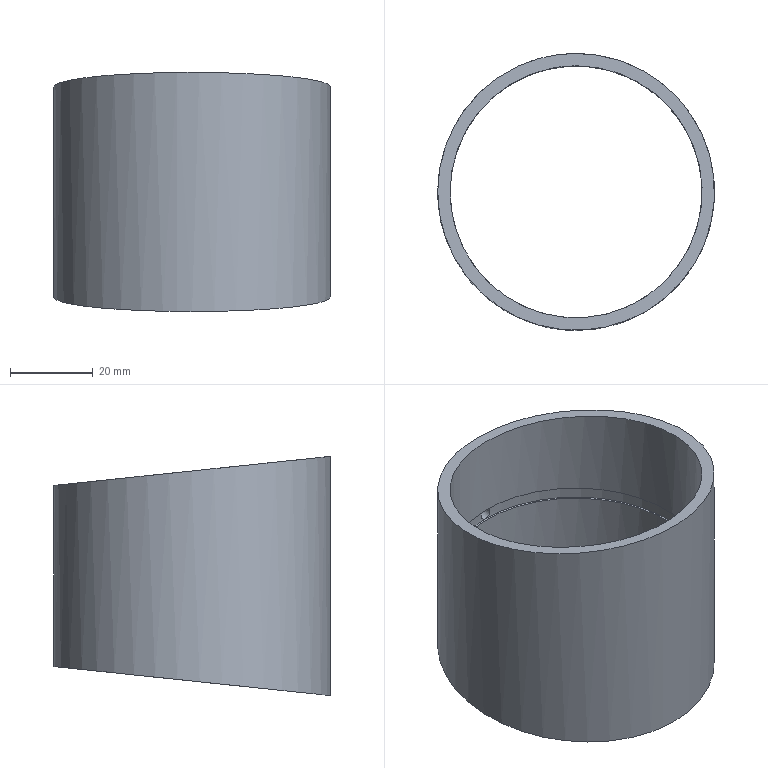Part | NX | features DATUM_CSYS 5, EXTRUDE 4, SKETCH 4, DATUM_PLANE 2, HOLE PACKAGE 1, MIRROR_SET 1, SIMPLE HOLE 1 | 1 solid | 9 faces | box 67 x 67 x 57.889 mm | volume 30363 mm3 | cylinder 5 | plane 4 | commonest cylinder face diameters 61 x2 3 x1 62 x1 67 x1
STEP:
#1=CARTESIAN_POINT('',(0.,30.5,52.218));
#2=VERTEX_POINT('',#1);
#3=CARTESIAN_POINT('',(0.,0.,55.423));
#4=DIRECTION('',(0.,-0.1045,-0.9945));
#5=DIRECTION('',(0.,0.9945,-0.1045));
#6=AXIS2_PLACEMENT_3D('',#3,#4,#5);
#7=ELLIPSE('',#6,30.668,30.5);
#8=EDGE_CURVE('',#2,#2,#7,.T.);
#9=ORIENTED_EDGE('',*,*,#8,.F.);
#10=EDGE_LOOP('',(#9));
#11=FACE_BOUND('',#10,.T.);
#12=CARTESIAN_POINT('',(-30.5,0.,32.));
#13=VERTEX_POINT('',#12);
#14=CARTESIAN_POINT('',(0.,0.,32.));
#15=DIRECTION('',(0.,0.,-1.));
#16=DIRECTION('',(-1.,0.,0.));
#17=AXIS2_PLACEMENT_3D('',#14,#15,#16);
#18=CIRCLE('',#17,30.5);
#19=EDGE_CURVE('',#13,#13,#18,.T.);
#20=ORIENTED_EDGE('',*,*,#19,.T.);
#21=EDGE_LOOP('',(#20));
#22=FACE_BOUND('',#21,.T.);
#23=CARTESIAN_POINT('',(0.,0.,60.));
#24=DIRECTION('',(0.,0.,-1.));
#25=DIRECTION('',(-1.,0.,0.));
#26=AXIS2_PLACEMENT_3D('',#23,#24,#25);
#27=CYLINDRICAL_SURFACE('',#26,30.5);
#28=ADVANCED_FACE('',(#11,#22),#27,.F.);
#29=CARTESIAN_POINT('',(1.5,33.466,30.5));
#30=VERTEX_POINT('',#29);
#31=CARTESIAN_POINT('',(1.174,33.483,29.323));
#32=CARTESIAN_POINT('',(1.663,33.458,30.5));
#33=CARTESIAN_POINT('',(1.175,33.483,31.676));
#34=CARTESIAN_POINT('',(0.001228,33.508,32.162));
#35=CARTESIAN_POINT('',(-1.175,33.483,31.676));
#36=CARTESIAN_POINT('',(-1.662,33.458,30.5));
#37=CARTESIAN_POINT('',(-1.177,33.483,29.326));
#38=CARTESIAN_POINT('',(-0.001751,33.508,28.838));
#39=CARTESIAN_POINT('',(1.174,33.483,29.323));
#40=CARTESIAN_POINT('',(1.663,33.458,30.5));
#41=CARTESIAN_POINT('',(1.175,33.483,31.676));
#42=B_SPLINE_CURVE_WITH_KNOTS('',3,(#31,#32,#33,#34,#35,#36,#37,#38,#39,#40,#41),.UNSPECIFIED.,.T.,.F.,(1,1,1,1,1,1,1,1,1,1,1,1,1,1,1),(-0.003517,-0.002345,-0.001172,0.,0.001172,0.002345,0.003517,0.00469,0.005862,0.007035,0.008207,0.009379,0.01055,0.01172,0.0129),.UNSPECIFIED.);
#43=EDGE_CURVE('',#30,#30,#42,.T.);
#44=ORIENTED_EDGE('',*,*,#43,.T.);
#45=EDGE_LOOP('',(#44));
#46=FACE_BOUND('',#45,.T.);
#47=CARTESIAN_POINT('',(0.,-33.5,1.056));
#48=VERTEX_POINT('',#47);
#49=CARTESIAN_POINT('',(0.,0.,4.577));
#50=DIRECTION('',(0.,-0.1045,0.9945));
#51=DIRECTION('',(0.,-0.9945,-0.1045));
#52=AXIS2_PLACEMENT_3D('',#49,#50,#51);
#53=ELLIPSE('',#52,33.685,33.5);
#54=EDGE_CURVE('',#48,#48,#53,.T.);
#55=ORIENTED_EDGE('',*,*,#54,.T.);
#56=EDGE_LOOP('',(#55));
#57=FACE_BOUND('',#56,.T.);
#58=CARTESIAN_POINT('',(0.,33.5,51.902));
#59=VERTEX_POINT('',#58);
#60=CARTESIAN_POINT('',(0.,0.,55.423));
#61=DIRECTION('',(0.,-0.1045,-0.9945));
#62=DIRECTION('',(0.,0.9945,-0.1045));
#63=AXIS2_PLACEMENT_3D('',#60,#61,#62);
#64=ELLIPSE('',#63,33.685,33.5);
#65=EDGE_CURVE('',#59,#59,#64,.T.);
#66=ORIENTED_EDGE('',*,*,#65,.T.);
#67=EDGE_LOOP('',(#66));
#68=FACE_BOUND('',#67,.T.);
#69=CARTESIAN_POINT('',(0.,0.,60.));
#70=DIRECTION('',(0.,0.,-1.));
#71=DIRECTION('',(-1.,0.,0.));
#72=AXIS2_PLACEMENT_3D('',#69,#70,#71);
#73=CYLINDRICAL_SURFACE('',#72,33.5);
#74=ADVANCED_FACE('',(#46,#57,#68),#73,.T.);
#75=CARTESIAN_POINT('',(-30.5,0.,29.));
#76=VERTEX_POINT('',#75);
#77=CARTESIAN_POINT('',(0.,0.,29.));
#78=DIRECTION('',(0.,0.,-1.));
#79=DIRECTION('',(-1.,0.,0.));
#80=AXIS2_PLACEMENT_3D('',#77,#78,#79);
#81=CIRCLE('',#80,30.5);
#82=EDGE_CURVE('',#76,#76,#81,.T.);
#83=ORIENTED_EDGE('',*,*,#82,.F.);
#84=EDGE_LOOP('',(#83));
#85=FACE_BOUND('',#84,.T.);
#86=CARTESIAN_POINT('',(0.,-30.5,1.371));
#87=VERTEX_POINT('',#86);
#88=CARTESIAN_POINT('',(0.,0.,4.577));
#89=DIRECTION('',(0.,-0.1045,0.9945));
#90=DIRECTION('',(0.,-0.9945,-0.1045));
#91=AXIS2_PLACEMENT_3D('',#88,#89,#90);
#92=ELLIPSE('',#91,30.668,30.5);
#93=EDGE_CURVE('',#87,#87,#92,.T.);
#94=ORIENTED_EDGE('',*,*,#93,.F.);
#95=EDGE_LOOP('',(#94));
#96=FACE_BOUND('',#95,.T.);
#97=CARTESIAN_POINT('',(0.,0.,60.));
#98=DIRECTION('',(0.,0.,-1.));
#99=DIRECTION('',(-1.,0.,0.));
#100=AXIS2_PLACEMENT_3D('',#97,#98,#99);
#101=CYLINDRICAL_SURFACE('',#100,30.5);
#102=ADVANCED_FACE('',(#85,#96),#101,.F.);
#103=ORIENTED_EDGE('',*,*,#8,.T.);
#104=EDGE_LOOP('',(#103));
#105=FACE_BOUND('',#104,.T.);
#106=ORIENTED_EDGE('',*,*,#65,.F.);
#107=EDGE_LOOP('',(#106));
#108=FACE_BOUND('',#107,.T.);
#109=CARTESIAN_POINT('',(-60.,-43.544,60.));
#110=DIRECTION('',(0.,-0.1045,-0.9945));
#111=DIRECTION('',(0.,0.9945,-0.1045));
#112=AXIS2_PLACEMENT_3D('',#109,#110,#111);
#113=PLANE('',#112);
#114=ADVANCED_FACE('',(#105,#108),#113,.F.);
#115=ORIENTED_EDGE('',*,*,#93,.T.);
#116=EDGE_LOOP('',(#115));
#117=FACE_BOUND('',#116,.T.);
#118=ORIENTED_EDGE('',*,*,#54,.F.);
#119=EDGE_LOOP('',(#118));
#120=FACE_BOUND('',#119,.T.);
#121=CARTESIAN_POINT('',(-60.,-43.544,0.));
#122=DIRECTION('',(0.,-0.1045,0.9945));
#123=DIRECTION('',(0.,0.9945,0.1045));
#124=AXIS2_PLACEMENT_3D('',#121,#122,#123);
#125=PLANE('',#124);
#126=ADVANCED_FACE('',(#117,#120),#125,.F.);
#127=CARTESIAN_POINT('',(0.,31.,29.));
#128=VERTEX_POINT('',#127);
#129=CARTESIAN_POINT('',(0.,31.,32.));
#130=VERTEX_POINT('',#129);
#131=CARTESIAN_POINT('',(0.,31.,29.));
#132=CARTESIAN_POINT('',(0.3958,31.,29.));
#133=CARTESIAN_POINT('',(1.174,30.982,29.324));
#134=CARTESIAN_POINT('',(1.663,30.955,30.502));
#135=CARTESIAN_POINT('',(1.174,30.982,31.676));
#136=CARTESIAN_POINT('',(0.3913,31.,32.));
#137=CARTESIAN_POINT('',(0.,31.,32.));
#138=B_SPLINE_CURVE_WITH_KNOTS('',3,(#131,#132,#133,#134,#135,#136,#137),.UNSPECIFIED.,.F.,.F.,(4,1,1,1,4),(0.007036,0.008209,0.009381,0.01055,0.01173),.UNSPECIFIED.);
#139=EDGE_CURVE('',#128,#130,#138,.T.);
#140=ORIENTED_EDGE('',*,*,#139,.T.);
#141=CARTESIAN_POINT('',(0.,31.,32.));
#142=CARTESIAN_POINT('',(-0.3914,31.,32.));
#143=CARTESIAN_POINT('',(-1.176,30.982,31.675));
#144=CARTESIAN_POINT('',(-1.663,30.955,30.499));
#145=CARTESIAN_POINT('',(-1.174,30.982,29.325));
#146=CARTESIAN_POINT('',(-0.3959,31.,29.));
#147=CARTESIAN_POINT('',(0.,31.,29.));
#148=B_SPLINE_CURVE_WITH_KNOTS('',3,(#141,#142,#143,#144,#145,#146,#147),.UNSPECIFIED.,.F.,.F.,(4,1,1,1,4),(0.002346,0.003518,0.004691,0.005864,0.007036),.UNSPECIFIED.);
#149=EDGE_CURVE('',#130,#128,#148,.T.);
#150=ORIENTED_EDGE('',*,*,#149,.T.);
#151=EDGE_LOOP('',(#140,#150));
#152=FACE_BOUND('',#151,.T.);
#153=ORIENTED_EDGE('',*,*,#43,.F.);
#154=EDGE_LOOP('',(#153));
#155=FACE_BOUND('',#154,.T.);
#156=CARTESIAN_POINT('',(0.,35.,30.5));
#157=DIRECTION('',(0.,-1.,0.));
#158=DIRECTION('',(1.,0.,0.));
#159=AXIS2_PLACEMENT_3D('',#156,#157,#158);
#160=CYLINDRICAL_SURFACE('',#159,1.5);
#161=ADVANCED_FACE('',(#152,#155),#160,.F.);
#162=CARTESIAN_POINT('',(0.,0.,32.));
#163=DIRECTION('',(0.,0.,-1.));
#164=DIRECTION('',(1.,0.,0.));
#165=AXIS2_PLACEMENT_3D('',#162,#163,#164);
#166=CIRCLE('',#165,31.);
#167=EDGE_CURVE('',#130,#130,#166,.F.);
#168=ORIENTED_EDGE('',*,*,#167,.T.);
#169=ORIENTED_EDGE('',*,*,#139,.F.);
#170=CARTESIAN_POINT('',(0.,0.,29.));
#171=DIRECTION('',(0.,0.,-1.));
#172=DIRECTION('',(1.,0.,0.));
#173=AXIS2_PLACEMENT_3D('',#170,#171,#172);
#174=CIRCLE('',#173,31.);
#175=EDGE_CURVE('',#128,#128,#174,.F.);
#176=ORIENTED_EDGE('',*,*,#175,.F.);
#177=ORIENTED_EDGE('',*,*,#149,.F.);
#178=EDGE_LOOP('',(#168,#169,#176,#177));
#179=FACE_BOUND('',#178,.T.);
#180=CARTESIAN_POINT('',(0.,0.,32.));
#181=DIRECTION('',(0.,0.,-1.));
#182=DIRECTION('',(-1.,0.,0.));
#183=AXIS2_PLACEMENT_3D('',#180,#181,#182);
#184=CYLINDRICAL_SURFACE('',#183,31.);
#185=ADVANCED_FACE('',(#179),#184,.F.);
#186=ORIENTED_EDGE('',*,*,#167,.F.);
#187=EDGE_LOOP('',(#186));
#188=FACE_BOUND('',#187,.T.);
#189=ORIENTED_EDGE('',*,*,#19,.F.);
#190=EDGE_LOOP('',(#189));
#191=FACE_BOUND('',#190,.T.);
#192=CARTESIAN_POINT('',(0.,0.,32.));
#193=DIRECTION('',(0.,0.,-1.));
#194=DIRECTION('',(-1.,0.,0.));
#195=AXIS2_PLACEMENT_3D('',#192,#193,#194);
#196=PLANE('',#195);
#197=ADVANCED_FACE('',(#188,#191),#196,.T.);
#198=ORIENTED_EDGE('',*,*,#175,.T.);
#199=EDGE_LOOP('',(#198));
#200=FACE_BOUND('',#199,.T.);
#201=ORIENTED_EDGE('',*,*,#82,.T.);
#202=EDGE_LOOP('',(#201));
#203=FACE_BOUND('',#202,.T.);
#204=CARTESIAN_POINT('',(0.,0.,29.));
#205=DIRECTION('',(0.,0.,-1.));
#206=DIRECTION('',(-1.,0.,0.));
#207=AXIS2_PLACEMENT_3D('',#204,#205,#206);
#208=PLANE('',#207);
#209=ADVANCED_FACE('',(#200,#203),#208,.F.);
#210=CLOSED_SHELL('',(#28,#74,#102,#114,#126,#161,#185,#197,#209));
#211=MANIFOLD_SOLID_BREP('',#210);
#212=(LENGTH_UNIT()NAMED_UNIT(*)SI_UNIT(.MILLI.,.METRE.));
#213=UNCERTAINTY_MEASURE_WITH_UNIT(LENGTH_MEASURE(0.0508),#212,'','');
#214=(NAMED_UNIT(*)PLANE_ANGLE_UNIT()SI_UNIT($,.RADIAN.));
#215=(NAMED_UNIT(*)SI_UNIT($,.STERADIAN.)SOLID_ANGLE_UNIT());
#216=(GEOMETRIC_REPRESENTATION_CONTEXT(3)GLOBAL_UNCERTAINTY_ASSIGNED_CONTEXT((#213))GLOBAL_UNIT_ASSIGNED_CONTEXT((#212,#214,#215))REPRESENTATION_CONTEXT('',''));
#217=ADVANCED_BREP_SHAPE_REPRESENTATION('',(#211),#216);